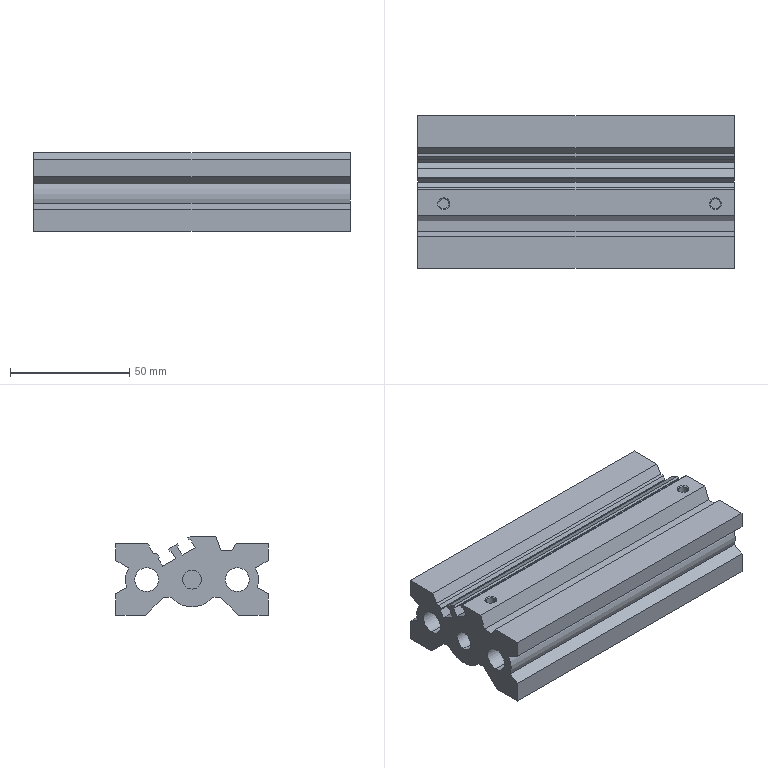Part | SolidWorks | features ICE 5, HoleWzd 4, LPattern 4, RefAxis 3, 3DProfileFeature 1, Extrusion 1, RevCut 1 | 1 solid | 111 faces | box 133 x 64 x 33 mm | volume 163699 mm3 | plane 44 | cone 36 | cylinder 31 | commonest cylinder face diameters 4.134 x20 10 x4 8 x2 16 x2 18 x2 23 x1